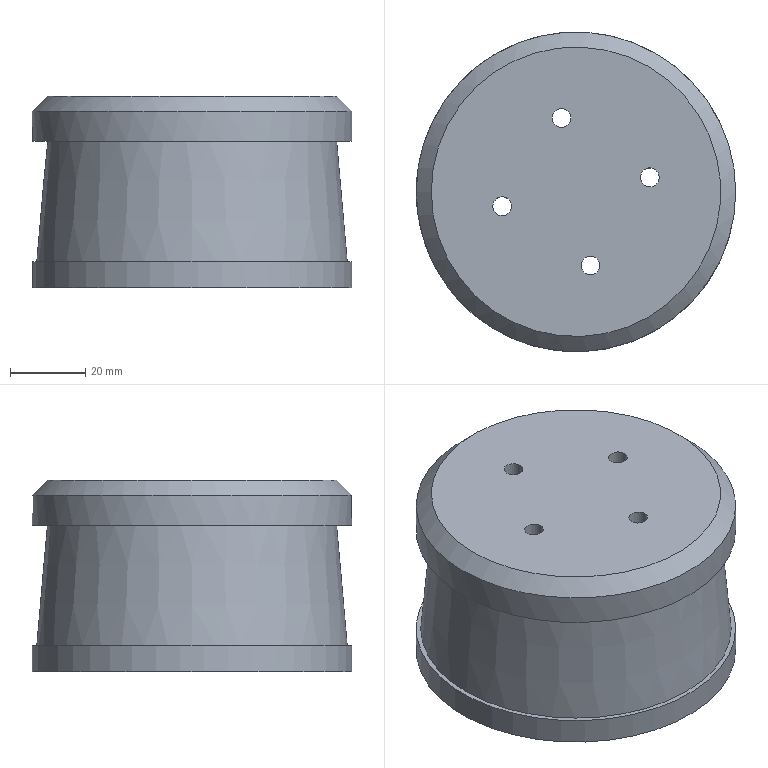Part | NX | features BREP 1 | 1 solid | 15 faces | box 85 x 85 x 51 mm | volume 144942 mm3 | cylinder 7 | plane 6 | cone 2 | commonest cylinder face diameters 5 x4 85 x2 59.433 x1
STEP:
#1=CARTESIAN_POINT('',(42.5,0.,-46.));
#2=VERTEX_POINT('',#1);
#3=CARTESIAN_POINT('',(0.,0.,-46.));
#4=DIRECTION('',(0.,0.,-1.));
#5=DIRECTION('',(1.,0.,0.));
#6=AXIS2_PLACEMENT_3D('',#3,#4,#5);
#7=CIRCLE('',#6,42.5);
#8=EDGE_CURVE('',#2,#2,#7,.T.);
#9=ORIENTED_EDGE('',*,*,#8,.F.);
#10=EDGE_LOOP('',(#9));
#11=FACE_BOUND('',#10,.T.);
#12=CARTESIAN_POINT('',(42.5,0.,-39.));
#13=VERTEX_POINT('',#12);
#14=CARTESIAN_POINT('',(0.,0.,-39.));
#15=DIRECTION('',(0.,0.,-1.));
#16=DIRECTION('',(1.,0.,0.));
#17=AXIS2_PLACEMENT_3D('',#14,#15,#16);
#18=CIRCLE('',#17,42.5);
#19=EDGE_CURVE('',#13,#13,#18,.T.);
#20=ORIENTED_EDGE('',*,*,#19,.T.);
#21=EDGE_LOOP('',(#20));
#22=FACE_BOUND('',#21,.T.);
#23=CARTESIAN_POINT('',(0.,0.,0.));
#24=DIRECTION('',(0.,0.,-1.));
#25=DIRECTION('',(1.,0.,0.));
#26=AXIS2_PLACEMENT_3D('',#23,#24,#25);
#27=CYLINDRICAL_SURFACE('',#26,42.5);
#28=ADVANCED_FACE('',(#11,#22),#27,.T.);
#29=CARTESIAN_POINT('',(-18.189,-23.5,-46.));
#30=VERTEX_POINT('',#29);
#31=CARTESIAN_POINT('',(18.189,-23.5,-46.));
#32=VERTEX_POINT('',#31);
#33=CARTESIAN_POINT('',(0.,0.,-46.));
#34=DIRECTION('',(0.,0.,-1.));
#35=DIRECTION('',(1.,0.,0.));
#36=AXIS2_PLACEMENT_3D('',#33,#34,#35);
#37=CIRCLE('',#36,29.717);
#38=EDGE_CURVE('',#30,#32,#37,.T.);
#39=ORIENTED_EDGE('',*,*,#38,.T.);
#40=CARTESIAN_POINT('',(18.189,-23.5,0.));
#41=VERTEX_POINT('',#40);
#42=CARTESIAN_POINT('',(18.189,-23.5,0.));
#43=DIRECTION('',(0.,0.,1.));
#44=VECTOR('',#43,1000.);
#45=LINE('',#42,#44);
#46=EDGE_CURVE('',#32,#41,#45,.T.);
#47=ORIENTED_EDGE('',*,*,#46,.T.);
#48=CARTESIAN_POINT('',(-18.189,-23.5,0.));
#49=VERTEX_POINT('',#48);
#50=CARTESIAN_POINT('',(0.,0.,0.));
#51=DIRECTION('',(0.,0.,-1.));
#52=DIRECTION('',(1.,0.,0.));
#53=AXIS2_PLACEMENT_3D('',#50,#51,#52);
#54=CIRCLE('',#53,29.717);
#55=EDGE_CURVE('',#49,#41,#54,.T.);
#56=ORIENTED_EDGE('',*,*,#55,.F.);
#57=CARTESIAN_POINT('',(-18.189,-23.5,0.));
#58=DIRECTION('',(0.,0.,-1.));
#59=VECTOR('',#58,1000.);
#60=LINE('',#57,#59);
#61=EDGE_CURVE('',#49,#30,#60,.T.);
#62=ORIENTED_EDGE('',*,*,#61,.T.);
#63=EDGE_LOOP('',(#39,#47,#56,#62));
#64=FACE_BOUND('',#63,.T.);
#65=CARTESIAN_POINT('',(0.,0.,0.));
#66=DIRECTION('',(0.,0.,-1.));
#67=DIRECTION('',(1.,0.,0.));
#68=AXIS2_PLACEMENT_3D('',#65,#66,#67);
#69=CYLINDRICAL_SURFACE('',#68,29.717);
#70=ADVANCED_FACE('',(#64),#69,.F.);
#71=CARTESIAN_POINT('',(42.5,0.,-7.));
#72=VERTEX_POINT('',#71);
#73=CARTESIAN_POINT('',(0.,0.,-7.));
#74=DIRECTION('',(0.,0.,-1.));
#75=DIRECTION('',(1.,0.,0.));
#76=AXIS2_PLACEMENT_3D('',#73,#74,#75);
#77=CIRCLE('',#76,42.5);
#78=EDGE_CURVE('',#72,#72,#77,.T.);
#79=ORIENTED_EDGE('',*,*,#78,.F.);
#80=EDGE_LOOP('',(#79));
#81=FACE_BOUND('',#80,.T.);
#82=CARTESIAN_POINT('',(-42.5,0.,1.));
#83=VERTEX_POINT('',#82);
#84=CARTESIAN_POINT('',(0.,0.,1.));
#85=DIRECTION('',(0.,0.,-1.));
#86=DIRECTION('',(-1.,0.,0.));
#87=AXIS2_PLACEMENT_3D('',#84,#85,#86);
#88=CIRCLE('',#87,42.5);
#89=EDGE_CURVE('',#83,#83,#88,.T.);
#90=ORIENTED_EDGE('',*,*,#89,.T.);
#91=EDGE_LOOP('',(#90));
#92=FACE_BOUND('',#91,.T.);
#93=CARTESIAN_POINT('',(0.,0.,0.));
#94=DIRECTION('',(0.,0.,-1.));
#95=DIRECTION('',(1.,0.,0.));
#96=AXIS2_PLACEMENT_3D('',#93,#94,#95);
#97=CYLINDRICAL_SURFACE('',#96,42.5);
#98=ADVANCED_FACE('',(#81,#92),#97,.T.);
#99=CARTESIAN_POINT('',(18.189,-23.5,-46.));
#100=DIRECTION('',(-1.,0.,0.));
#101=VECTOR('',#100,1000.);
#102=LINE('',#99,#101);
#103=EDGE_CURVE('',#32,#30,#102,.T.);
#104=ORIENTED_EDGE('',*,*,#103,.T.);
#105=ORIENTED_EDGE('',*,*,#61,.F.);
#106=CARTESIAN_POINT('',(18.189,-23.5,0.));
#107=DIRECTION('',(-1.,0.,0.));
#108=VECTOR('',#107,1000.);
#109=LINE('',#106,#108);
#110=EDGE_CURVE('',#41,#49,#109,.T.);
#111=ORIENTED_EDGE('',*,*,#110,.F.);
#112=ORIENTED_EDGE('',*,*,#46,.F.);
#113=EDGE_LOOP('',(#104,#105,#111,#112));
#114=FACE_BOUND('',#113,.T.);
#115=CARTESIAN_POINT('',(18.189,-23.5,0.));
#116=DIRECTION('',(0.,-1.,0.));
#117=DIRECTION('',(-1.,0.,0.));
#118=AXIS2_PLACEMENT_3D('',#115,#116,#117);
#119=PLANE('',#118);
#120=ADVANCED_FACE('',(#114),#119,.F.);
#121=ORIENTED_EDGE('',*,*,#8,.T.);
#122=EDGE_LOOP('',(#121));
#123=FACE_BOUND('',#122,.T.);
#124=ORIENTED_EDGE('',*,*,#38,.F.);
#125=ORIENTED_EDGE('',*,*,#103,.F.);
#126=EDGE_LOOP('',(#124,#125));
#127=FACE_BOUND('',#126,.T.);
#128=CARTESIAN_POINT('',(0.,0.,-46.));
#129=DIRECTION('',(0.,0.,-1.));
#130=DIRECTION('',(1.,0.,0.));
#131=AXIS2_PLACEMENT_3D('',#128,#129,#130);
#132=PLANE('',#131);
#133=ADVANCED_FACE('',(#123,#127),#132,.T.);
#134=CARTESIAN_POINT('',(17.126,3.848,0.));
#135=VERTEX_POINT('',#134);
#136=CARTESIAN_POINT('',(19.626,3.848,0.));
#137=DIRECTION('',(0.,0.,-1.));
#138=DIRECTION('',(-1.,0.,0.));
#139=AXIS2_PLACEMENT_3D('',#136,#137,#138);
#140=CIRCLE('',#139,2.5);
#141=EDGE_CURVE('',#135,#135,#140,.T.);
#142=ORIENTED_EDGE('',*,*,#141,.F.);
#143=EDGE_LOOP('',(#142));
#144=FACE_BOUND('',#143,.T.);
#145=CARTESIAN_POINT('',(1.348,-19.626,0.));
#146=VERTEX_POINT('',#145);
#147=CARTESIAN_POINT('',(3.848,-19.626,0.));
#148=DIRECTION('',(0.,0.,-1.));
#149=DIRECTION('',(-1.,0.,0.));
#150=AXIS2_PLACEMENT_3D('',#147,#148,#149);
#151=CIRCLE('',#150,2.5);
#152=EDGE_CURVE('',#146,#146,#151,.T.);
#153=ORIENTED_EDGE('',*,*,#152,.F.);
#154=EDGE_LOOP('',(#153));
#155=FACE_BOUND('',#154,.T.);
#156=CARTESIAN_POINT('',(-6.348,19.626,0.));
#157=VERTEX_POINT('',#156);
#158=CARTESIAN_POINT('',(-3.848,19.626,0.));
#159=DIRECTION('',(0.,0.,-1.));
#160=DIRECTION('',(-1.,0.,0.));
#161=AXIS2_PLACEMENT_3D('',#158,#159,#160);
#162=CIRCLE('',#161,2.5);
#163=EDGE_CURVE('',#157,#157,#162,.T.);
#164=ORIENTED_EDGE('',*,*,#163,.F.);
#165=EDGE_LOOP('',(#164));
#166=FACE_BOUND('',#165,.T.);
#167=CARTESIAN_POINT('',(-22.126,-3.848,0.));
#168=VERTEX_POINT('',#167);
#169=CARTESIAN_POINT('',(-19.626,-3.848,0.));
#170=DIRECTION('',(0.,0.,-1.));
#171=DIRECTION('',(-1.,0.,0.));
#172=AXIS2_PLACEMENT_3D('',#169,#170,#171);
#173=CIRCLE('',#172,2.5);
#174=EDGE_CURVE('',#168,#168,#173,.T.);
#175=ORIENTED_EDGE('',*,*,#174,.F.);
#176=EDGE_LOOP('',(#175));
#177=FACE_BOUND('',#176,.T.);
#178=ORIENTED_EDGE('',*,*,#110,.T.);
#179=ORIENTED_EDGE('',*,*,#55,.T.);
#180=EDGE_LOOP('',(#178,#179));
#181=FACE_BOUND('',#180,.T.);
#182=CARTESIAN_POINT('',(0.,0.,0.));
#183=DIRECTION('',(0.,0.,-1.));
#184=DIRECTION('',(1.,0.,0.));
#185=AXIS2_PLACEMENT_3D('',#182,#183,#184);
#186=PLANE('',#185);
#187=ADVANCED_FACE('',(#144,#155,#166,#177,#181),#186,.T.);
#188=CARTESIAN_POINT('',(17.126,3.848,5.));
#189=VERTEX_POINT('',#188);
#190=CARTESIAN_POINT('',(19.626,3.848,5.));
#191=DIRECTION('',(0.,0.,-1.));
#192=DIRECTION('',(-1.,0.,0.));
#193=AXIS2_PLACEMENT_3D('',#190,#191,#192);
#194=CIRCLE('',#193,2.5);
#195=EDGE_CURVE('',#189,#189,#194,.T.);
#196=ORIENTED_EDGE('',*,*,#195,.T.);
#197=EDGE_LOOP('',(#196));
#198=FACE_BOUND('',#197,.T.);
#199=CARTESIAN_POINT('',(1.348,-19.626,5.));
#200=VERTEX_POINT('',#199);
#201=CARTESIAN_POINT('',(3.848,-19.626,5.));
#202=DIRECTION('',(0.,0.,-1.));
#203=DIRECTION('',(-1.,0.,0.));
#204=AXIS2_PLACEMENT_3D('',#201,#202,#203);
#205=CIRCLE('',#204,2.5);
#206=EDGE_CURVE('',#200,#200,#205,.T.);
#207=ORIENTED_EDGE('',*,*,#206,.T.);
#208=EDGE_LOOP('',(#207));
#209=FACE_BOUND('',#208,.T.);
#210=CARTESIAN_POINT('',(-6.348,19.626,5.));
#211=VERTEX_POINT('',#210);
#212=CARTESIAN_POINT('',(-3.848,19.626,5.));
#213=DIRECTION('',(0.,0.,-1.));
#214=DIRECTION('',(-1.,0.,0.));
#215=AXIS2_PLACEMENT_3D('',#212,#213,#214);
#216=CIRCLE('',#215,2.5);
#217=EDGE_CURVE('',#211,#211,#216,.T.);
#218=ORIENTED_EDGE('',*,*,#217,.T.);
#219=EDGE_LOOP('',(#218));
#220=FACE_BOUND('',#219,.T.);
#221=CARTESIAN_POINT('',(-22.126,-3.848,5.));
#222=VERTEX_POINT('',#221);
#223=CARTESIAN_POINT('',(-19.626,-3.848,5.));
#224=DIRECTION('',(0.,0.,-1.));
#225=DIRECTION('',(-1.,0.,0.));
#226=AXIS2_PLACEMENT_3D('',#223,#224,#225);
#227=CIRCLE('',#226,2.5);
#228=EDGE_CURVE('',#222,#222,#227,.T.);
#229=ORIENTED_EDGE('',*,*,#228,.T.);
#230=EDGE_LOOP('',(#229));
#231=FACE_BOUND('',#230,.T.);
#232=CARTESIAN_POINT('',(-38.5,0.,5.));
#233=VERTEX_POINT('',#232);
#234=CARTESIAN_POINT('',(0.,0.,5.));
#235=DIRECTION('',(0.,0.,1.));
#236=DIRECTION('',(-1.,0.,0.));
#237=AXIS2_PLACEMENT_3D('',#234,#235,#236);
#238=CIRCLE('',#237,38.5);
#239=EDGE_CURVE('',#233,#233,#238,.T.);
#240=ORIENTED_EDGE('',*,*,#239,.T.);
#241=EDGE_LOOP('',(#240));
#242=FACE_BOUND('',#241,.T.);
#243=CARTESIAN_POINT('',(0.,0.,5.));
#244=DIRECTION('',(0.,0.,-1.));
#245=DIRECTION('',(1.,0.,0.));
#246=AXIS2_PLACEMENT_3D('',#243,#244,#245);
#247=PLANE('',#246);
#248=ADVANCED_FACE('',(#198,#209,#220,#231,#242),#247,.F.);
#249=ORIENTED_EDGE('',*,*,#239,.F.);
#250=EDGE_LOOP('',(#249));
#251=FACE_BOUND('',#250,.T.);
#252=ORIENTED_EDGE('',*,*,#89,.F.);
#253=EDGE_LOOP('',(#252));
#254=FACE_BOUND('',#253,.T.);
#255=CARTESIAN_POINT('',(0.,0.,1.));
#256=DIRECTION('',(0.,0.,-1.));
#257=DIRECTION('',(1.,0.,0.));
#258=AXIS2_PLACEMENT_3D('',#255,#256,#257);
#259=CONICAL_SURFACE('',#258,42.5,0.7854);
#260=ADVANCED_FACE('',(#251,#254),#259,.T.);
#261=ORIENTED_EDGE('',*,*,#174,.T.);
#262=EDGE_LOOP('',(#261));
#263=FACE_BOUND('',#262,.T.);
#264=ORIENTED_EDGE('',*,*,#228,.F.);
#265=EDGE_LOOP('',(#264));
#266=FACE_BOUND('',#265,.T.);
#267=CARTESIAN_POINT('',(-19.626,-3.848,-63.));
#268=DIRECTION('',(0.,0.,1.));
#269=DIRECTION('',(-1.,0.,0.));
#270=AXIS2_PLACEMENT_3D('',#267,#268,#269);
#271=CYLINDRICAL_SURFACE('',#270,2.5);
#272=ADVANCED_FACE('',(#263,#266),#271,.F.);
#273=ORIENTED_EDGE('',*,*,#163,.T.);
#274=EDGE_LOOP('',(#273));
#275=FACE_BOUND('',#274,.T.);
#276=ORIENTED_EDGE('',*,*,#217,.F.);
#277=EDGE_LOOP('',(#276));
#278=FACE_BOUND('',#277,.T.);
#279=CARTESIAN_POINT('',(-3.848,19.626,-63.));
#280=DIRECTION('',(0.,0.,1.));
#281=DIRECTION('',(-1.,0.,0.));
#282=AXIS2_PLACEMENT_3D('',#279,#280,#281);
#283=CYLINDRICAL_SURFACE('',#282,2.5);
#284=ADVANCED_FACE('',(#275,#278),#283,.F.);
#285=ORIENTED_EDGE('',*,*,#152,.T.);
#286=EDGE_LOOP('',(#285));
#287=FACE_BOUND('',#286,.T.);
#288=ORIENTED_EDGE('',*,*,#206,.F.);
#289=EDGE_LOOP('',(#288));
#290=FACE_BOUND('',#289,.T.);
#291=CARTESIAN_POINT('',(3.848,-19.626,-63.));
#292=DIRECTION('',(0.,0.,1.));
#293=DIRECTION('',(-1.,0.,0.));
#294=AXIS2_PLACEMENT_3D('',#291,#292,#293);
#295=CYLINDRICAL_SURFACE('',#294,2.5);
#296=ADVANCED_FACE('',(#287,#290),#295,.F.);
#297=ORIENTED_EDGE('',*,*,#141,.T.);
#298=EDGE_LOOP('',(#297));
#299=FACE_BOUND('',#298,.T.);
#300=ORIENTED_EDGE('',*,*,#195,.F.);
#301=EDGE_LOOP('',(#300));
#302=FACE_BOUND('',#301,.T.);
#303=CARTESIAN_POINT('',(19.626,3.848,-63.));
#304=DIRECTION('',(0.,0.,1.));
#305=DIRECTION('',(-1.,0.,0.));
#306=AXIS2_PLACEMENT_3D('',#303,#304,#305);
#307=CYLINDRICAL_SURFACE('',#306,2.5);
#308=ADVANCED_FACE('',(#299,#302),#307,.F.);
#309=CARTESIAN_POINT('',(41.3,0.,-39.));
#310=VERTEX_POINT('',#309);
#311=CARTESIAN_POINT('',(0.,0.,-39.));
#312=DIRECTION('',(0.,0.,-1.));
#313=DIRECTION('',(1.,0.,0.));
#314=AXIS2_PLACEMENT_3D('',#311,#312,#313);
#315=CIRCLE('',#314,41.3);
#316=EDGE_CURVE('',#310,#310,#315,.T.);
#317=ORIENTED_EDGE('',*,*,#316,.F.);
#318=EDGE_LOOP('',(#317));
#319=FACE_BOUND('',#318,.T.);
#320=CARTESIAN_POINT('',(38.5,0.,-7.));
#321=VERTEX_POINT('',#320);
#322=CARTESIAN_POINT('',(0.,0.,-7.));
#323=DIRECTION('',(0.,0.,-1.));
#324=DIRECTION('',(1.,0.,0.));
#325=AXIS2_PLACEMENT_3D('',#322,#323,#324);
#326=CIRCLE('',#325,38.5);
#327=EDGE_CURVE('',#321,#321,#326,.T.);
#328=ORIENTED_EDGE('',*,*,#327,.T.);
#329=EDGE_LOOP('',(#328));
#330=FACE_BOUND('',#329,.T.);
#331=CARTESIAN_POINT('',(0.,0.,-7.));
#332=DIRECTION('',(0.,0.,-1.));
#333=DIRECTION('',(-1.,0.,0.));
#334=AXIS2_PLACEMENT_3D('',#331,#332,#333);
#335=CONICAL_SURFACE('',#334,38.5,0.08727);
#336=ADVANCED_FACE('',(#319,#330),#335,.T.);
#337=ORIENTED_EDGE('',*,*,#19,.F.);
#338=EDGE_LOOP('',(#337));
#339=FACE_BOUND('',#338,.T.);
#340=ORIENTED_EDGE('',*,*,#316,.T.);
#341=EDGE_LOOP('',(#340));
#342=FACE_BOUND('',#341,.T.);
#343=CARTESIAN_POINT('',(0.,0.,-39.));
#344=DIRECTION('',(0.,0.,1.));
#345=DIRECTION('',(-1.,0.,0.));
#346=AXIS2_PLACEMENT_3D('',#343,#344,#345);
#347=PLANE('',#346);
#348=ADVANCED_FACE('',(#339,#342),#347,.T.);
#349=ORIENTED_EDGE('',*,*,#78,.T.);
#350=EDGE_LOOP('',(#349));
#351=FACE_BOUND('',#350,.T.);
#352=ORIENTED_EDGE('',*,*,#327,.F.);
#353=EDGE_LOOP('',(#352));
#354=FACE_BOUND('',#353,.T.);
#355=CARTESIAN_POINT('',(0.,0.,-7.));
#356=DIRECTION('',(0.,0.,1.));
#357=DIRECTION('',(-1.,0.,0.));
#358=AXIS2_PLACEMENT_3D('',#355,#356,#357);
#359=PLANE('',#358);
#360=ADVANCED_FACE('',(#351,#354),#359,.F.);
#361=CLOSED_SHELL('',(#28,#70,#98,#120,#133,#187,#248,#260,#272,#284,#296,#308,#336,#348,#360));
#362=MANIFOLD_SOLID_BREP('',#361);
#363=(LENGTH_UNIT()NAMED_UNIT(*)SI_UNIT(.MILLI.,.METRE.));
#364=UNCERTAINTY_MEASURE_WITH_UNIT(LENGTH_MEASURE(0.00001),#363,'','');
#365=(NAMED_UNIT(*)PLANE_ANGLE_UNIT()SI_UNIT($,.RADIAN.));
#366=(NAMED_UNIT(*)SI_UNIT($,.STERADIAN.)SOLID_ANGLE_UNIT());
#367=(GEOMETRIC_REPRESENTATION_CONTEXT(3)GLOBAL_UNCERTAINTY_ASSIGNED_CONTEXT((#364))GLOBAL_UNIT_ASSIGNED_CONTEXT((#363,#365,#366))REPRESENTATION_CONTEXT('',''));
#368=ADVANCED_BREP_SHAPE_REPRESENTATION('',(#362),#367);